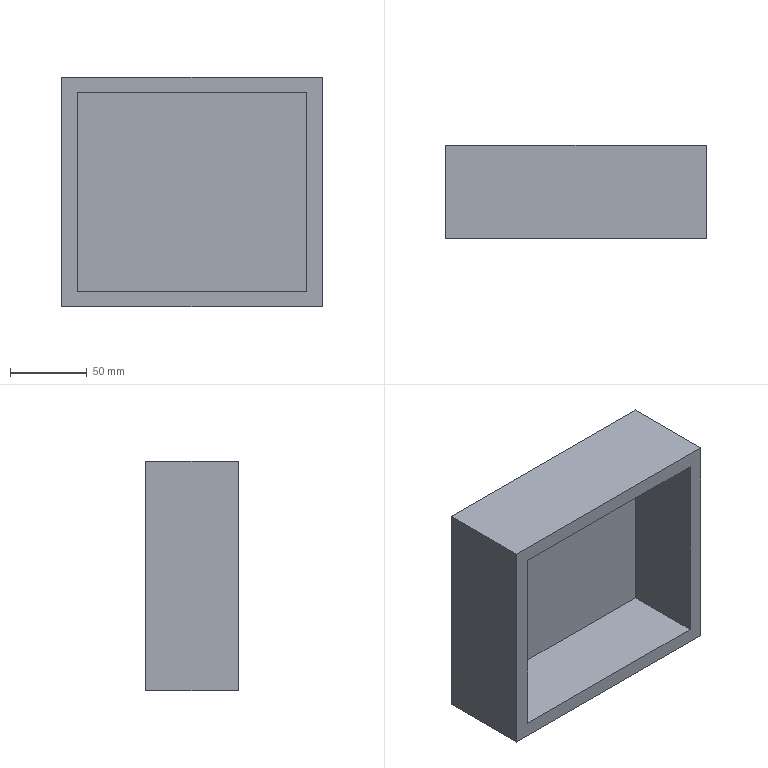Part | SolidWorks | features Extrusion 1, ICE 1 | 1 solid | 11 faces | box 170 x 60.52 x 150 mm | volume 558120 mm3 | plane 11
STEP:
#1=CARTESIAN_POINT('',(-117.516,35.221,0.));
#2=VERTEX_POINT('',#1);
#3=CARTESIAN_POINT('',(-117.516,-25.299,0.));
#4=VERTEX_POINT('',#3);
#5=CARTESIAN_POINT('',(-117.516,35.221,0.));
#6=DIRECTION('',(0.,-1.,0.));
#7=VECTOR('',#6,1000.);
#8=LINE('',#5,#7);
#9=EDGE_CURVE('',#2,#4,#8,.T.);
#10=ORIENTED_EDGE('',*,*,#9,.T.);
#11=CARTESIAN_POINT('',(-117.516,-25.299,150.));
#12=VERTEX_POINT('',#11);
#13=CARTESIAN_POINT('',(-117.516,-25.299,150.));
#14=DIRECTION('',(0.,0.,-1.));
#15=VECTOR('',#14,1000.);
#16=LINE('',#13,#15);
#17=EDGE_CURVE('',#12,#4,#16,.T.);
#18=ORIENTED_EDGE('',*,*,#17,.F.);
#19=CARTESIAN_POINT('',(-117.516,35.221,150.));
#20=VERTEX_POINT('',#19);
#21=CARTESIAN_POINT('',(-117.516,35.221,150.));
#22=DIRECTION('',(0.,-1.,0.));
#23=VECTOR('',#22,1000.);
#24=LINE('',#21,#23);
#25=EDGE_CURVE('',#20,#12,#24,.T.);
#26=ORIENTED_EDGE('',*,*,#25,.F.);
#27=CARTESIAN_POINT('',(-117.516,35.221,150.));
#28=DIRECTION('',(0.,0.,-1.));
#29=VECTOR('',#28,1000.);
#30=LINE('',#27,#29);
#31=EDGE_CURVE('',#20,#2,#30,.T.);
#32=ORIENTED_EDGE('',*,*,#31,.T.);
#33=EDGE_LOOP('',(#10,#18,#26,#32));
#34=FACE_OUTER_BOUND('',#33,.T.);
#35=CARTESIAN_POINT('',(-117.516,35.221,150.));
#36=DIRECTION('',(1.,0.,0.));
#37=DIRECTION('',(0.,0.,-1.));
#38=AXIS2_PLACEMENT_3D('',#35,#36,#37);
#39=PLANE('',#38);
#40=ADVANCED_FACE('',(#34),#39,.F.);
#41=CARTESIAN_POINT('',(-107.516,-25.299,10.));
#42=VERTEX_POINT('',#41);
#43=CARTESIAN_POINT('',(42.484,-25.299,10.));
#44=VERTEX_POINT('',#43);
#45=CARTESIAN_POINT('',(-107.516,-25.299,10.));
#46=DIRECTION('',(1.,0.,0.));
#47=VECTOR('',#46,1000.);
#48=LINE('',#45,#47);
#49=EDGE_CURVE('',#42,#44,#48,.T.);
#50=ORIENTED_EDGE('',*,*,#49,.F.);
#51=CARTESIAN_POINT('',(-107.516,-25.299,140.));
#52=VERTEX_POINT('',#51);
#53=CARTESIAN_POINT('',(-107.516,-25.299,140.));
#54=DIRECTION('',(0.,0.,-1.));
#55=VECTOR('',#54,1000.);
#56=LINE('',#53,#55);
#57=EDGE_CURVE('',#52,#42,#56,.T.);
#58=ORIENTED_EDGE('',*,*,#57,.F.);
#59=CARTESIAN_POINT('',(42.484,-25.299,140.));
#60=VERTEX_POINT('',#59);
#61=CARTESIAN_POINT('',(-107.516,-25.299,140.));
#62=DIRECTION('',(-1.,0.,0.));
#63=VECTOR('',#62,1000.);
#64=LINE('',#61,#63);
#65=EDGE_CURVE('',#60,#52,#64,.T.);
#66=ORIENTED_EDGE('',*,*,#65,.F.);
#67=CARTESIAN_POINT('',(42.484,-25.299,140.));
#68=DIRECTION('',(0.,0.,1.));
#69=VECTOR('',#68,1000.);
#70=LINE('',#67,#69);
#71=EDGE_CURVE('',#44,#60,#70,.T.);
#72=ORIENTED_EDGE('',*,*,#71,.F.);
#73=EDGE_LOOP('',(#50,#58,#66,#72));
#74=FACE_BOUND('',#73,.T.);
#75=CARTESIAN_POINT('',(52.484,-25.299,0.));
#76=VERTEX_POINT('',#75);
#77=CARTESIAN_POINT('',(-117.516,-25.299,0.));
#78=DIRECTION('',(1.,0.,0.));
#79=VECTOR('',#78,1000.);
#80=LINE('',#77,#79);
#81=EDGE_CURVE('',#4,#76,#80,.T.);
#82=ORIENTED_EDGE('',*,*,#81,.T.);
#83=CARTESIAN_POINT('',(52.484,-25.299,150.));
#84=VERTEX_POINT('',#83);
#85=CARTESIAN_POINT('',(52.484,-25.299,150.));
#86=DIRECTION('',(0.,0.,-1.));
#87=VECTOR('',#86,1000.);
#88=LINE('',#85,#87);
#89=EDGE_CURVE('',#84,#76,#88,.T.);
#90=ORIENTED_EDGE('',*,*,#89,.F.);
#91=CARTESIAN_POINT('',(-117.516,-25.299,150.));
#92=DIRECTION('',(1.,0.,0.));
#93=VECTOR('',#92,1000.);
#94=LINE('',#91,#93);
#95=EDGE_CURVE('',#12,#84,#94,.T.);
#96=ORIENTED_EDGE('',*,*,#95,.F.);
#97=ORIENTED_EDGE('',*,*,#17,.T.);
#98=EDGE_LOOP('',(#82,#90,#96,#97));
#99=FACE_OUTER_BOUND('',#98,.T.);
#100=CARTESIAN_POINT('',(-117.516,-25.299,150.));
#101=DIRECTION('',(0.,1.,0.));
#102=DIRECTION('',(0.,0.,1.));
#103=AXIS2_PLACEMENT_3D('',#100,#101,#102);
#104=PLANE('',#103);
#105=ADVANCED_FACE('',(#74,#99),#104,.F.);
#106=CARTESIAN_POINT('',(52.484,35.221,0.));
#107=VERTEX_POINT('',#106);
#108=CARTESIAN_POINT('',(52.484,35.221,0.));
#109=DIRECTION('',(0.,1.,0.));
#110=VECTOR('',#109,1000.);
#111=LINE('',#108,#110);
#112=EDGE_CURVE('',#76,#107,#111,.T.);
#113=ORIENTED_EDGE('',*,*,#112,.T.);
#114=CARTESIAN_POINT('',(52.484,35.221,150.));
#115=VERTEX_POINT('',#114);
#116=CARTESIAN_POINT('',(52.484,35.221,150.));
#117=DIRECTION('',(0.,0.,-1.));
#118=VECTOR('',#117,1000.);
#119=LINE('',#116,#118);
#120=EDGE_CURVE('',#115,#107,#119,.T.);
#121=ORIENTED_EDGE('',*,*,#120,.F.);
#122=CARTESIAN_POINT('',(52.484,35.221,150.));
#123=DIRECTION('',(0.,1.,0.));
#124=VECTOR('',#123,1000.);
#125=LINE('',#122,#124);
#126=EDGE_CURVE('',#84,#115,#125,.T.);
#127=ORIENTED_EDGE('',*,*,#126,.F.);
#128=ORIENTED_EDGE('',*,*,#89,.T.);
#129=EDGE_LOOP('',(#113,#121,#127,#128));
#130=FACE_OUTER_BOUND('',#129,.T.);
#131=CARTESIAN_POINT('',(52.484,35.221,150.));
#132=DIRECTION('',(-1.,0.,0.));
#133=DIRECTION('',(0.,0.,1.));
#134=AXIS2_PLACEMENT_3D('',#131,#132,#133);
#135=PLANE('',#134);
#136=ADVANCED_FACE('',(#130),#135,.F.);
#137=CARTESIAN_POINT('',(-117.516,35.221,0.));
#138=DIRECTION('',(-1.,0.,0.));
#139=VECTOR('',#138,1000.);
#140=LINE('',#137,#139);
#141=EDGE_CURVE('',#107,#2,#140,.T.);
#142=ORIENTED_EDGE('',*,*,#141,.T.);
#143=ORIENTED_EDGE('',*,*,#31,.F.);
#144=CARTESIAN_POINT('',(-117.516,35.221,150.));
#145=DIRECTION('',(-1.,0.,0.));
#146=VECTOR('',#145,1000.);
#147=LINE('',#144,#146);
#148=EDGE_CURVE('',#115,#20,#147,.T.);
#149=ORIENTED_EDGE('',*,*,#148,.F.);
#150=ORIENTED_EDGE('',*,*,#120,.T.);
#151=EDGE_LOOP('',(#142,#143,#149,#150));
#152=FACE_OUTER_BOUND('',#151,.T.);
#153=CARTESIAN_POINT('',(-117.516,35.221,150.));
#154=DIRECTION('',(0.,-1.,0.));
#155=DIRECTION('',(1.,0.,0.));
#156=AXIS2_PLACEMENT_3D('',#153,#154,#155);
#157=PLANE('',#156);
#158=ADVANCED_FACE('',(#152),#157,.F.);
#159=ORIENTED_EDGE('',*,*,#25,.T.);
#160=ORIENTED_EDGE('',*,*,#95,.T.);
#161=ORIENTED_EDGE('',*,*,#126,.T.);
#162=ORIENTED_EDGE('',*,*,#148,.T.);
#163=EDGE_LOOP('',(#159,#160,#161,#162));
#164=FACE_OUTER_BOUND('',#163,.T.);
#165=CARTESIAN_POINT('',(0.,0.,150.));
#166=DIRECTION('',(0.,0.,1.));
#167=DIRECTION('',(1.,0.,0.));
#168=AXIS2_PLACEMENT_3D('',#165,#166,#167);
#169=PLANE('',#168);
#170=ADVANCED_FACE('',(#164),#169,.T.);
#171=ORIENTED_EDGE('',*,*,#9,.F.);
#172=ORIENTED_EDGE('',*,*,#141,.F.);
#173=ORIENTED_EDGE('',*,*,#112,.F.);
#174=ORIENTED_EDGE('',*,*,#81,.F.);
#175=EDGE_LOOP('',(#171,#172,#173,#174));
#176=FACE_OUTER_BOUND('',#175,.T.);
#177=CARTESIAN_POINT('',(0.,0.,0.));
#178=DIRECTION('',(0.,0.,1.));
#179=DIRECTION('',(1.,0.,0.));
#180=AXIS2_PLACEMENT_3D('',#177,#178,#179);
#181=PLANE('',#180);
#182=ADVANCED_FACE('',(#176),#181,.F.);
#183=ORIENTED_EDGE('',*,*,#57,.T.);
#184=CARTESIAN_POINT('',(-107.516,25.221,10.));
#185=VERTEX_POINT('',#184);
#186=CARTESIAN_POINT('',(-107.516,25.221,10.));
#187=DIRECTION('',(0.,-1.,0.));
#188=VECTOR('',#187,1000.);
#189=LINE('',#186,#188);
#190=EDGE_CURVE('',#185,#42,#189,.T.);
#191=ORIENTED_EDGE('',*,*,#190,.F.);
#192=CARTESIAN_POINT('',(-107.516,25.221,140.));
#193=VERTEX_POINT('',#192);
#194=CARTESIAN_POINT('',(-107.516,25.221,140.));
#195=DIRECTION('',(0.,0.,-1.));
#196=VECTOR('',#195,1000.);
#197=LINE('',#194,#196);
#198=EDGE_CURVE('',#193,#185,#197,.T.);
#199=ORIENTED_EDGE('',*,*,#198,.F.);
#200=CARTESIAN_POINT('',(-107.516,25.221,140.));
#201=DIRECTION('',(0.,-1.,0.));
#202=VECTOR('',#201,1000.);
#203=LINE('',#200,#202);
#204=EDGE_CURVE('',#193,#52,#203,.T.);
#205=ORIENTED_EDGE('',*,*,#204,.T.);
#206=EDGE_LOOP('',(#183,#191,#199,#205));
#207=FACE_OUTER_BOUND('',#206,.T.);
#208=CARTESIAN_POINT('',(-107.516,25.221,140.));
#209=DIRECTION('',(-1.,0.,0.));
#210=DIRECTION('',(0.,0.,1.));
#211=AXIS2_PLACEMENT_3D('',#208,#209,#210);
#212=PLANE('',#211);
#213=ADVANCED_FACE('',(#207),#212,.F.);
#214=ORIENTED_EDGE('',*,*,#65,.T.);
#215=ORIENTED_EDGE('',*,*,#204,.F.);
#216=CARTESIAN_POINT('',(42.484,25.221,140.));
#217=VERTEX_POINT('',#216);
#218=CARTESIAN_POINT('',(-107.516,25.221,140.));
#219=DIRECTION('',(-1.,0.,0.));
#220=VECTOR('',#219,1000.);
#221=LINE('',#218,#220);
#222=EDGE_CURVE('',#217,#193,#221,.T.);
#223=ORIENTED_EDGE('',*,*,#222,.F.);
#224=CARTESIAN_POINT('',(42.484,25.221,140.));
#225=DIRECTION('',(0.,-1.,0.));
#226=VECTOR('',#225,1000.);
#227=LINE('',#224,#226);
#228=EDGE_CURVE('',#217,#60,#227,.T.);
#229=ORIENTED_EDGE('',*,*,#228,.T.);
#230=EDGE_LOOP('',(#214,#215,#223,#229));
#231=FACE_OUTER_BOUND('',#230,.T.);
#232=CARTESIAN_POINT('',(-107.516,25.221,140.));
#233=DIRECTION('',(0.,0.,1.));
#234=DIRECTION('',(1.,0.,0.));
#235=AXIS2_PLACEMENT_3D('',#232,#233,#234);
#236=PLANE('',#235);
#237=ADVANCED_FACE('',(#231),#236,.F.);
#238=ORIENTED_EDGE('',*,*,#71,.T.);
#239=ORIENTED_EDGE('',*,*,#228,.F.);
#240=CARTESIAN_POINT('',(42.484,25.221,10.));
#241=VERTEX_POINT('',#240);
#242=CARTESIAN_POINT('',(42.484,25.221,140.));
#243=DIRECTION('',(0.,0.,1.));
#244=VECTOR('',#243,1000.);
#245=LINE('',#242,#244);
#246=EDGE_CURVE('',#241,#217,#245,.T.);
#247=ORIENTED_EDGE('',*,*,#246,.F.);
#248=CARTESIAN_POINT('',(42.484,25.221,10.));
#249=DIRECTION('',(0.,-1.,0.));
#250=VECTOR('',#249,1000.);
#251=LINE('',#248,#250);
#252=EDGE_CURVE('',#241,#44,#251,.T.);
#253=ORIENTED_EDGE('',*,*,#252,.T.);
#254=EDGE_LOOP('',(#238,#239,#247,#253));
#255=FACE_OUTER_BOUND('',#254,.T.);
#256=CARTESIAN_POINT('',(42.484,25.221,140.));
#257=DIRECTION('',(1.,0.,0.));
#258=DIRECTION('',(0.,0.,-1.));
#259=AXIS2_PLACEMENT_3D('',#256,#257,#258);
#260=PLANE('',#259);
#261=ADVANCED_FACE('',(#255),#260,.F.);
#262=ORIENTED_EDGE('',*,*,#49,.T.);
#263=ORIENTED_EDGE('',*,*,#252,.F.);
#264=CARTESIAN_POINT('',(-107.516,25.221,10.));
#265=DIRECTION('',(1.,0.,0.));
#266=VECTOR('',#265,1000.);
#267=LINE('',#264,#266);
#268=EDGE_CURVE('',#185,#241,#267,.T.);
#269=ORIENTED_EDGE('',*,*,#268,.F.);
#270=ORIENTED_EDGE('',*,*,#190,.T.);
#271=EDGE_LOOP('',(#262,#263,#269,#270));
#272=FACE_OUTER_BOUND('',#271,.T.);
#273=CARTESIAN_POINT('',(-107.516,25.221,10.));
#274=DIRECTION('',(0.,0.,-1.));
#275=DIRECTION('',(-1.,0.,0.));
#276=AXIS2_PLACEMENT_3D('',#273,#274,#275);
#277=PLANE('',#276);
#278=ADVANCED_FACE('',(#272),#277,.F.);
#279=ORIENTED_EDGE('',*,*,#198,.T.);
#280=ORIENTED_EDGE('',*,*,#268,.T.);
#281=ORIENTED_EDGE('',*,*,#246,.T.);
#282=ORIENTED_EDGE('',*,*,#222,.T.);
#283=EDGE_LOOP('',(#279,#280,#281,#282));
#284=FACE_OUTER_BOUND('',#283,.T.);
#285=CARTESIAN_POINT('',(0.,25.221,0.));
#286=DIRECTION('',(0.,-1.,0.));
#287=DIRECTION('',(0.,0.,-1.));
#288=AXIS2_PLACEMENT_3D('',#285,#286,#287);
#289=PLANE('',#288);
#290=ADVANCED_FACE('',(#284),#289,.T.);
#291=CLOSED_SHELL('',(#40,#105,#136,#158,#170,#182,#213,#237,#261,#278,#290));
#292=MANIFOLD_SOLID_BREP('',#291);
#293=CARTESIAN_POINT('',(0.,0.,0.));
#294=DIRECTION('',(0.,0.,1.));
#295=DIRECTION('',(1.,0.,0.));
#296=AXIS2_PLACEMENT_3D('',#293,#294,#295);
#297=(LENGTH_UNIT()NAMED_UNIT(*)SI_UNIT(.MILLI.,.METRE.));
#298=UNCERTAINTY_MEASURE_WITH_UNIT(LENGTH_MEASURE(0.00001),#297,'','');
#299=(NAMED_UNIT(*)PLANE_ANGLE_UNIT()SI_UNIT($,.RADIAN.));
#300=(NAMED_UNIT(*)SI_UNIT($,.STERADIAN.)SOLID_ANGLE_UNIT());
#301=(GEOMETRIC_REPRESENTATION_CONTEXT(3)GLOBAL_UNCERTAINTY_ASSIGNED_CONTEXT((#298))GLOBAL_UNIT_ASSIGNED_CONTEXT((#297,#299,#300))REPRESENTATION_CONTEXT('',''));
#302=ADVANCED_BREP_SHAPE_REPRESENTATION('',(#292,#296),#301);